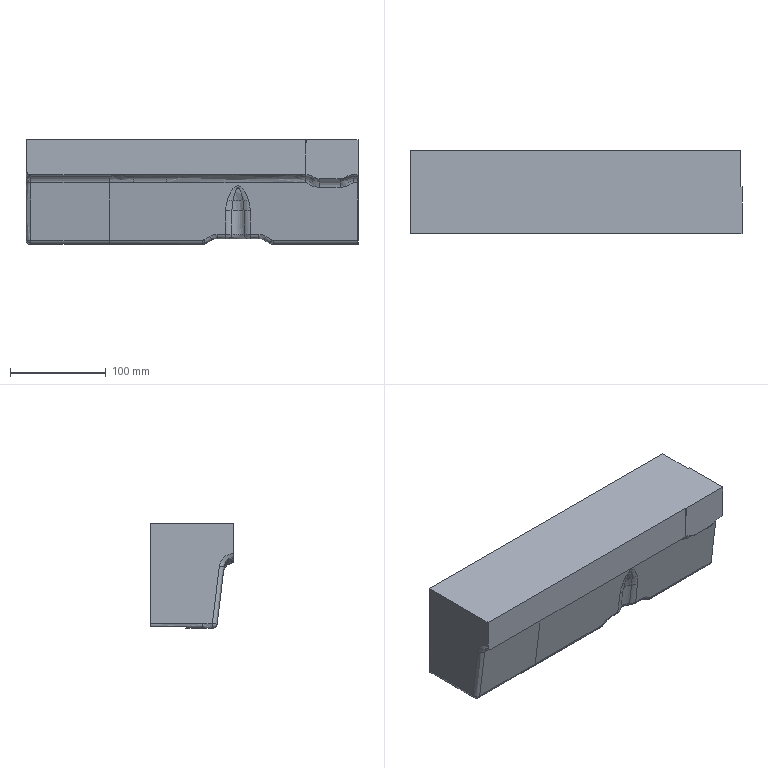Part | NX | features solid 2 | 1 solid | 110 faces | box 347.1 x 86.948 x 109.55 mm | volume 2900735 mm3 | spline 88 | plane 21 | sphere 1